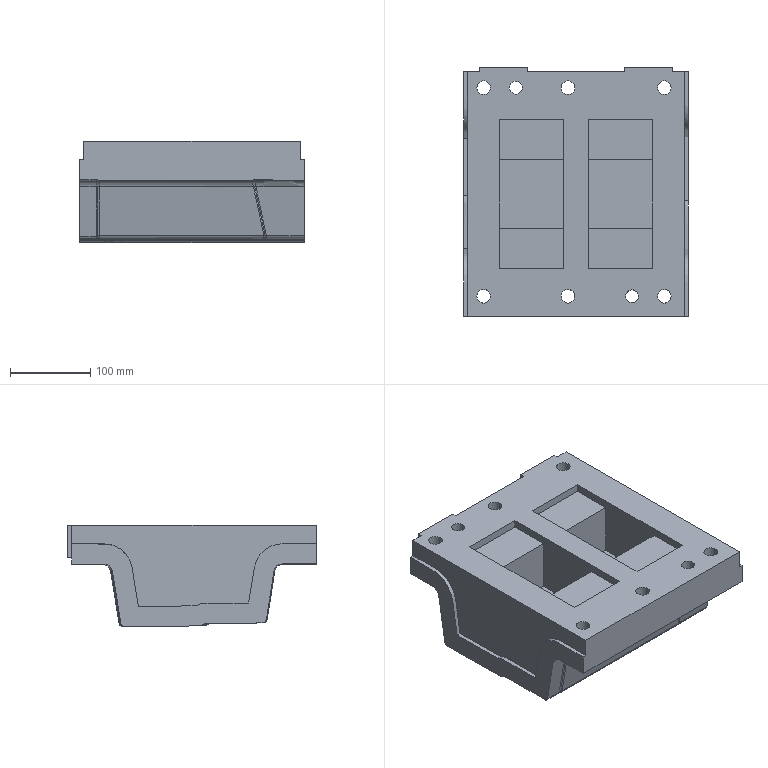Part | NX | features solid 2 | 1 solid | 157 faces | box 280 x 310 x 126.004 mm | volume 6791703 mm3 | spline 58 | plane 56 | cylinder 41 | sphere 1 | cone 1 | commonest cylinder face diameters 10 x7 8 x6 12 x6 17 x6 26 x6 20 x5